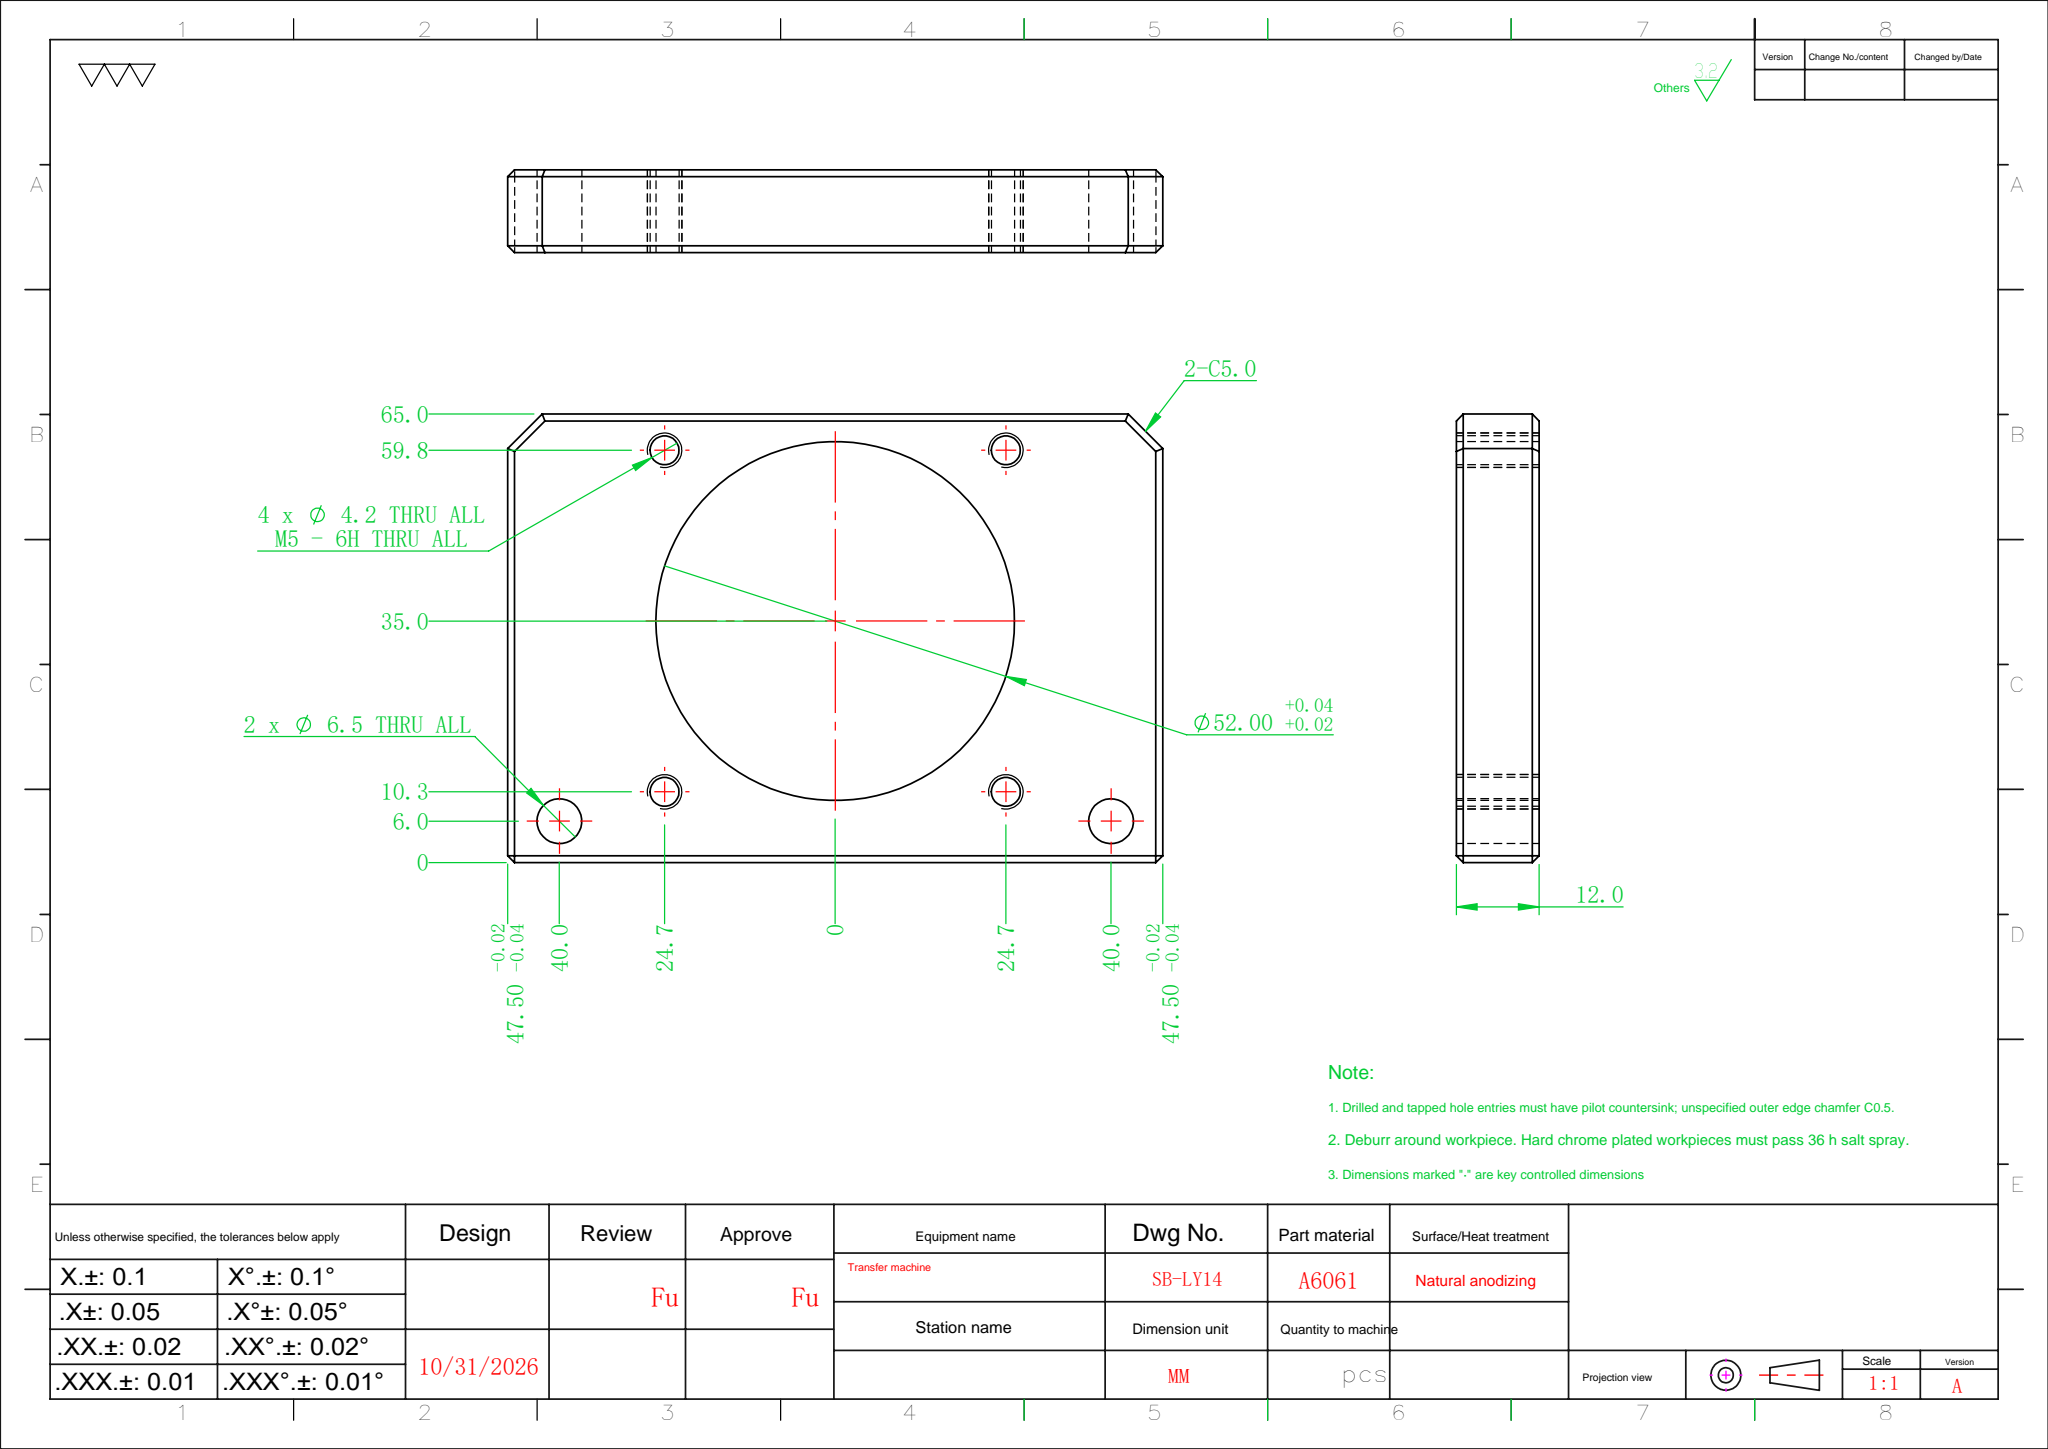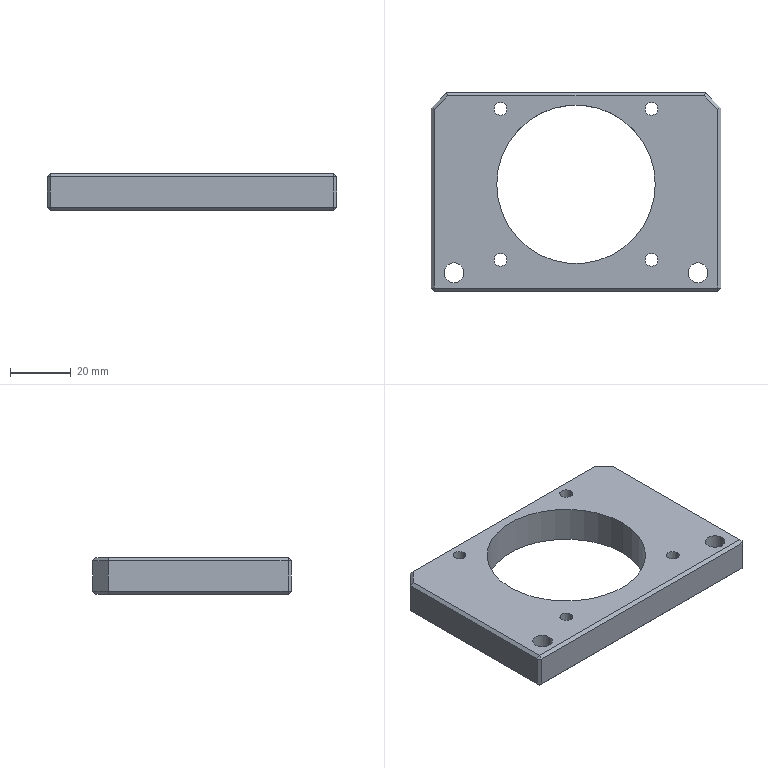Part | SolidWorks | features Chamfer 2, HoleWzd 2, Cut 1, Extrusion 1 | 1 solid | 40 faces | box 95 x 65 x 12 mm | volume 46532 mm3 | plane 26 | cylinder 14 | commonest cylinder face diameters 4.2 x8 6.5 x4 52 x2